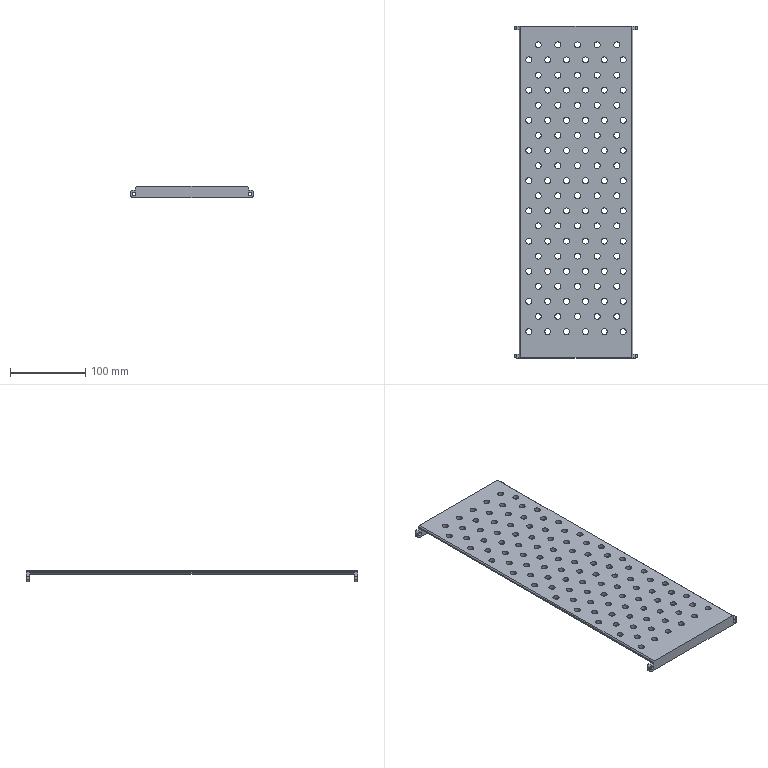Part | SolidWorks | features ICE 4, Chamfer 1, Extrusion 1, Fillet 1, LPattern 1 | 1 solid | 258 faces | box 163 x 440 x 15 mm | volume 316227 mm3 | cylinder 236 | plane 22 | commonest cylinder face diameters 8 x220 5 x8 6 x8